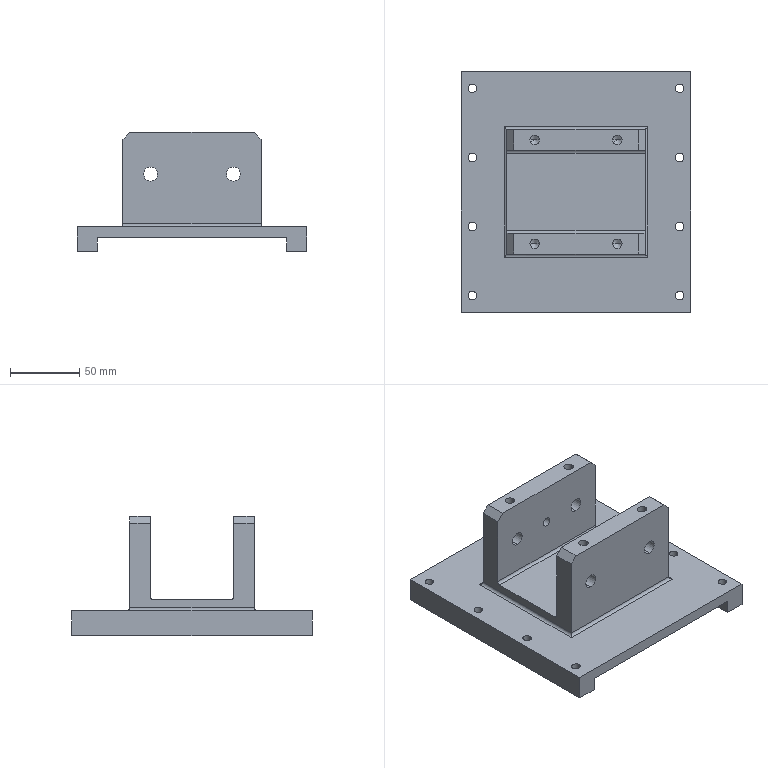NC program | NX | posted with a generic post | part box 166 x 174 x 86.2 mm
Lines 6608 to 6801 of 6801:
(FLOOR_WALL_2 , TOOL : D16-48-D16-100-3T-FINISH)
N13214 T02 M6
N13216 G54
N13218 G17 G0 G90 X98. Y72.5 S2500 M3
N13220 G43 Z30. H2
N13222 Z3.
N13224 G94 G1 Z0. F1000.
N13226 X95.
N13228 X-95.
N13230 Y76.6
N13232 X95.
N13234 X98.
N13236 Z3.
N13238 G0 Z30.
N13240 Y-79.
N13242 Z3.
N13244 G1 Z0.
N13246 X95.
N13248 X-95.
N13250 Y-74.9
N13252 X95.
N13254 X98.
N13256 Z3.
N13258 G0 Z30.
(FLOOR_WALL_2_COPY , TOOL : D16-48-D16-100-3T-FINISH)
N13260 X98.15 Y-60.347
N13262 Z-7.
N13264 G1 Z-10.
N13266 X95.
N13268 X-95.
N13270 Y-49.375
N13272 X95.
N13274 Y-38.402
N13276 X-95.
N13278 Y-27.43
N13280 X95.
N13282 Y-16.457
N13284 X-95.
N13286 Y-5.485
N13288 X95.
N13290 Y5.488
N13292 X-95.
N13294 Y16.46
N13296 X95.
N13298 Y27.433
N13300 X-95.
N13302 Y38.405
N13304 X95.
N13306 Y49.378
N13308 X-95.
N13310 Y60.35
N13312 X95.
N13314 X98.15
N13316 Z-7.
N13318 G0 Z30.
(FLOOR_WALL_2_COPY_COPY , TOOL : D16-48-D16-100-3T-FINISH)
N13320 X98. Y60.5
N13322 Z-7.
N13324 G1 Z-10.
N13326 X83.
N13328 X-83.
N13330 X-98.
N13332 Z-7.
N13334 G0 Z30.
N13336 Y-60.5
N13338 Z-7.
N13340 G1 Z-10.
N13342 X-83.
N13344 X83.
N13346 X98.
N13348 Z-7.
N13350 G0 Z30.
(PLANAR_MILL_6 , TOOL : D16-48-D16-100-3T-FINISH)
N13352 X-95.174 Y-97.841 S3000
N13354 Z-17.
N13356 G1 Z-20. F800.
N13358 G41 X-95. Y-96.856 D2
N13360 Y-82.997
N13362 Y83.
N13364 G2 X-87. Y91. R8.
N13366 G1 X87.
N13368 G2 X95. Y83. R8.
N13370 G1 Y-83.
N13372 G2 X87. Y-91. R8.
N13374 G1 X-86.997
N13376 X-100.856
N13378 G40
N13380 X-101.841 Y-91.174
N13382 Z-17.
N13384 G0 Z30.
N13386 M5
(DRILLING_1 , TOOL : 倒角D10-90度)
N13388 T03 M6
N13390 G54
N13392 G17 G0 G90 X-75. Y75. S1200 M3
N13394 G43 Z30. H3
N13396 G94 G81 G98 Z-3.2 F100. R3.
N13398 X-25.
N13400 X25.
N13402 X75.
N13404 Y-75.
N13406 X25.
N13408 X-25.
N13410 X-75.
N13412 G80
N13414 G0 X-75. Y-75. Z30.
N13416 M5
(DRILLING_1_COPY , TOOL : 钻头D6.5-73-105)
N13418 T08 M6
N13420 G54
N13422 G17 G0 G90 X-75. Y75. S1200 M3
N13424 G43 Z30. H8
N13426 G94 G83 G98 Z-25. F100. Q2. R3.
N13428 X-25.
N13430 X25.
N13432 X75.
N13434 Y-75.
N13436 X25.
N13438 X-25.
N13440 X-75.
N13442 G80
N13444 G0 X-75. Y-75. Z30.
N13446 M5
(PLANAR_MILL_4 , TOOL : 倒角D10-90度)
N13448 T03 M6
N13450 G54
N13452 G17 G0 G90 X-2. Y87. S3000 M3
N13454 G43 Z30. H3
N13456 Z0.
N13458 G94 G1 Z-2. F1000.
N13460 G3 X0. Y85. R2.
N13462 G1 X87.
N13464 G2 X89. Y83. R2.
N13466 G1 Y68.5
N13468 G2 X87. Y66.5 R2.
N13470 G1 X-87.
N13472 G2 X-89. Y68.5 R2.
N13474 G1 Y83.
N13476 G2 X-87. Y85. R2.
N13478 G1 X0.
N13480 G3 X2. Y87. R2.
N13482 G1 Z0.
N13484 G0 Z30.
N13486 Y-87.
N13488 Z0.
N13490 G1 Z-2.
N13492 G3 X0. Y-85. R2.
N13494 G1 X-87.
N13496 G2 X-89. Y-83. R2.
N13498 G1 Y-68.5
N13500 G2 X-87. Y-66.5 R2.
N13502 G1 X87.
N13504 G2 X89. Y-68.5 R2.
N13506 G1 Y-83.
N13508 G2 X87. Y-85. R2.
N13510 G1 X0.
N13512 G3 X-2. Y-87. R2.
N13514 G1 Z0.
N13516 G0 Z30.
(PLANAR_MILL_5 , TOOL : 倒角D10-90度)
N13518 X-92. Y-63.5
N13520 Z-11.
N13522 G1 Z-13.
N13524 G3 X-90. Y-61.5 R2.
N13526 G1 Y61.5
N13528 G3 X-92. Y63.5 R2.
N13530 G1 Z-11.
N13532 G0 Z30.
N13534 X92.
N13536 Z-11.
N13538 G1 Z-13.
N13540 G3 X90. Y61.5 R2.
N13542 G1 Y-61.5
N13544 G3 X92. Y-63.5 R2.
N13546 G1 Z-11.
N13548 G0 Z30.
N13550 M5
N13552 M2